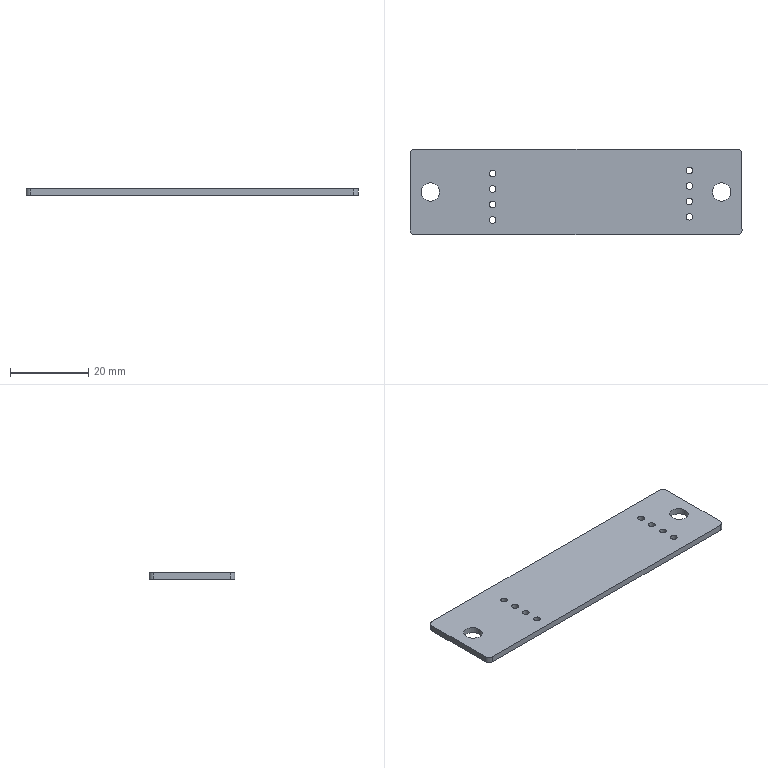Part | STEP file | SOLID | 1 solid | 20 faces | box 85 x 22 x 1.6 mm | volume 2905 mm3 | cylinder 14 | plane 6 | commonest cylinder face diameters 1.7 x8 2.54 x4 4.7 x2